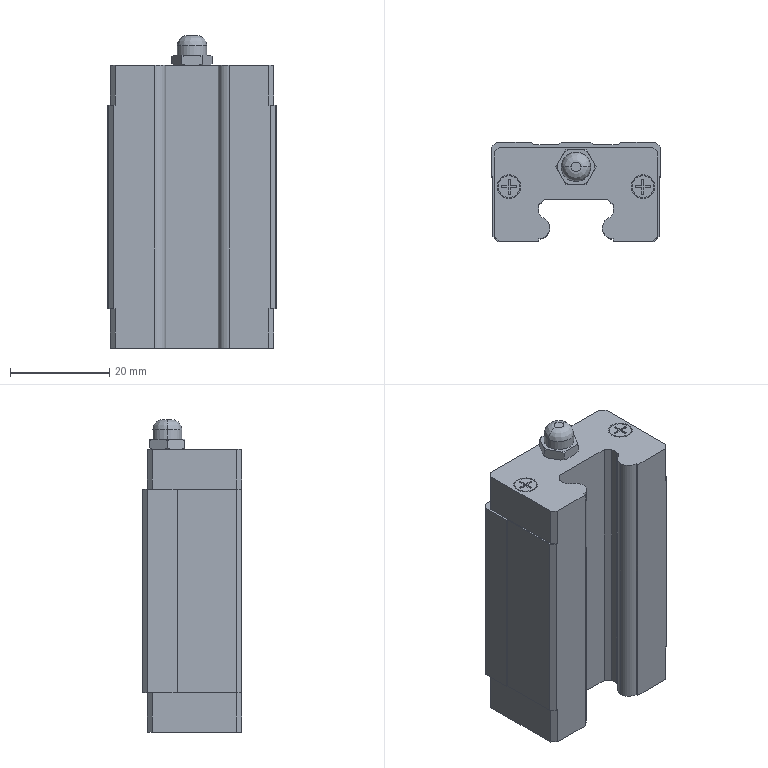Part | STEP file | block_SXR24 | 1 solid | 181 faces | box 34 x 20 x 63 mm | volume 30781 mm3 | plane 98 | cylinder 51 | cone 30 | other 2 | commonest cylinder face diameters 3.08 x20 4.4 x11 3.242 x8 4.8 x8 3 x2 5.94 x2